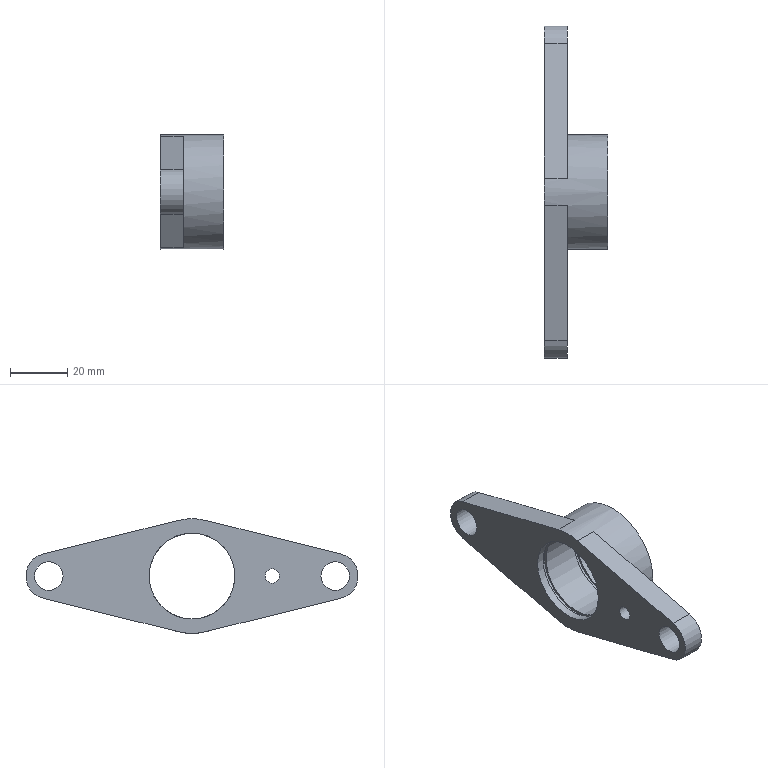Part | NX | features DATUM_CSYS 3, EXTRACT_FACE 2, EXTRUDE 2, RECT_GROOVE 2, Instance Feature 1, Mirror Feature 1, SKETCH 1 | 1 solid | 23 faces | box 22 x 116 x 40 mm | volume 25110 mm3 | plane 12 | cylinder 11 | commonest cylinder face diameters 30 x3 10 x2 16 x2 31.4 x2 5 x1 40 x1
STEP:
#1=CARTESIAN_POINT('',(22.,0.,15.));
#2=VERTEX_POINT('',#1);
#3=CARTESIAN_POINT('',(22.,0.,0.));
#4=DIRECTION('',(-1.,0.,0.));
#5=DIRECTION('',(0.,0.,1.));
#6=AXIS2_PLACEMENT_3D('',#3,#4,#5);
#7=CIRCLE('',#6,15.);
#8=EDGE_CURVE('',#2,#2,#7,.F.);
#9=ORIENTED_EDGE('',*,*,#8,.T.);
#10=EDGE_LOOP('',(#9));
#11=FACE_BOUND('',#10,.T.);
#12=CARTESIAN_POINT('',(19.2,0.,15.));
#13=VERTEX_POINT('',#12);
#14=CARTESIAN_POINT('',(19.2,0.,0.));
#15=DIRECTION('',(-1.,0.,0.));
#16=DIRECTION('',(0.,0.,1.));
#17=AXIS2_PLACEMENT_3D('',#14,#15,#16);
#18=CIRCLE('',#17,15.);
#19=EDGE_CURVE('',#13,#13,#18,.T.);
#20=ORIENTED_EDGE('',*,*,#19,.T.);
#21=EDGE_LOOP('',(#20));
#22=FACE_BOUND('',#21,.T.);
#23=CARTESIAN_POINT('',(8.,0.,0.));
#24=DIRECTION('',(-1.,0.,0.));
#25=DIRECTION('',(0.,0.,1.));
#26=AXIS2_PLACEMENT_3D('',#23,#24,#25);
#27=CYLINDRICAL_SURFACE('',#26,15.);
#28=ADVANCED_FACE('',(#11,#22),#27,.F.);
#29=CARTESIAN_POINT('',(0.,15.,0.));
#30=VERTEX_POINT('',#29);
#31=CARTESIAN_POINT('',(0.,0.,0.));
#32=DIRECTION('',(1.,0.,0.));
#33=DIRECTION('',(0.,1.,0.));
#34=AXIS2_PLACEMENT_3D('',#31,#32,#33);
#35=CIRCLE('',#34,15.);
#36=EDGE_CURVE('',#30,#30,#35,.T.);
#37=ORIENTED_EDGE('',*,*,#36,.F.);
#38=EDGE_LOOP('',(#37));
#39=FACE_BOUND('',#38,.T.);
#40=CARTESIAN_POINT('',(2.8,0.,-15.));
#41=VERTEX_POINT('',#40);
#42=CARTESIAN_POINT('',(2.8,0.,0.));
#43=DIRECTION('',(1.,0.,0.));
#44=DIRECTION('',(0.,0.,-1.));
#45=AXIS2_PLACEMENT_3D('',#42,#43,#44);
#46=CIRCLE('',#45,15.);
#47=EDGE_CURVE('',#41,#41,#46,.T.);
#48=ORIENTED_EDGE('',*,*,#47,.T.);
#49=EDGE_LOOP('',(#48));
#50=FACE_BOUND('',#49,.T.);
#51=CARTESIAN_POINT('',(8.,0.,0.));
#52=DIRECTION('',(-1.,0.,0.));
#53=DIRECTION('',(0.,0.,1.));
#54=AXIS2_PLACEMENT_3D('',#51,#52,#53);
#55=CYLINDRICAL_SURFACE('',#54,15.);
#56=ADVANCED_FACE('',(#39,#50),#55,.F.);
#57=CARTESIAN_POINT('',(8.,-25.5,0.));
#58=VERTEX_POINT('',#57);
#59=CARTESIAN_POINT('',(8.,-28.,0.));
#60=DIRECTION('',(1.,0.,0.));
#61=DIRECTION('',(0.,1.,0.));
#62=AXIS2_PLACEMENT_3D('',#59,#60,#61);
#63=CIRCLE('',#62,2.5);
#64=EDGE_CURVE('',#58,#58,#63,.T.);
#65=ORIENTED_EDGE('',*,*,#64,.F.);
#66=EDGE_LOOP('',(#65));
#67=FACE_BOUND('',#66,.T.);
#68=CARTESIAN_POINT('',(8.,-45.,0.));
#69=VERTEX_POINT('',#68);
#70=CARTESIAN_POINT('',(8.,-50.,0.));
#71=DIRECTION('',(1.,0.,0.));
#72=DIRECTION('',(0.,1.,0.));
#73=AXIS2_PLACEMENT_3D('',#70,#71,#72);
#74=CIRCLE('',#73,5.);
#75=EDGE_CURVE('',#69,#69,#74,.T.);
#76=ORIENTED_EDGE('',*,*,#75,.F.);
#77=EDGE_LOOP('',(#76));
#78=FACE_BOUND('',#77,.T.);
#79=CARTESIAN_POINT('',(8.,-4.8,19.415));
#80=VERTEX_POINT('',#79);
#81=CARTESIAN_POINT('',(8.,-4.8,-19.415));
#82=VERTEX_POINT('',#81);
#83=CARTESIAN_POINT('',(8.,0.,0.));
#84=DIRECTION('',(-1.,0.,0.));
#85=DIRECTION('',(0.,0.,1.));
#86=AXIS2_PLACEMENT_3D('',#83,#84,#85);
#87=CIRCLE('',#86,20.);
#88=EDGE_CURVE('',#80,#82,#87,.F.);
#89=ORIENTED_EDGE('',*,*,#88,.F.);
#90=CARTESIAN_POINT('',(8.,-51.92,7.766));
#91=VERTEX_POINT('',#90);
#92=CARTESIAN_POINT('',(8.,-51.92,7.766));
#93=DIRECTION('',(0.,0.9708,0.24));
#94=VECTOR('',#93,1000.);
#95=LINE('',#92,#94);
#96=EDGE_CURVE('',#91,#80,#95,.T.);
#97=ORIENTED_EDGE('',*,*,#96,.F.);
#98=CARTESIAN_POINT('',(8.,-51.92,-7.766));
#99=VERTEX_POINT('',#98);
#100=CARTESIAN_POINT('',(8.,-50.,0.));
#101=DIRECTION('',(-1.,0.,0.));
#102=DIRECTION('',(0.,1.,0.));
#103=AXIS2_PLACEMENT_3D('',#100,#101,#102);
#104=CIRCLE('',#103,8.);
#105=EDGE_CURVE('',#99,#91,#104,.T.);
#106=ORIENTED_EDGE('',*,*,#105,.F.);
#107=CARTESIAN_POINT('',(8.,-4.8,-19.415));
#108=DIRECTION('',(0.,-0.9708,0.24));
#109=VECTOR('',#108,1000.);
#110=LINE('',#107,#109);
#111=EDGE_CURVE('',#82,#99,#110,.T.);
#112=ORIENTED_EDGE('',*,*,#111,.F.);
#113=EDGE_LOOP('',(#89,#97,#106,#112));
#114=FACE_BOUND('',#113,.T.);
#115=CARTESIAN_POINT('',(8.,0.,0.));
#116=DIRECTION('',(-1.,0.,0.));
#117=DIRECTION('',(0.,0.,1.));
#118=AXIS2_PLACEMENT_3D('',#115,#116,#117);
#119=PLANE('',#118);
#120=ADVANCED_FACE('',(#67,#78,#114),#119,.F.);
#121=CARTESIAN_POINT('',(8.,45.,0.));
#122=VERTEX_POINT('',#121);
#123=CARTESIAN_POINT('',(8.,50.,0.));
#124=DIRECTION('',(-1.,0.,0.));
#125=DIRECTION('',(0.,-1.,0.));
#126=AXIS2_PLACEMENT_3D('',#123,#124,#125);
#127=CIRCLE('',#126,5.);
#128=EDGE_CURVE('',#122,#122,#127,.T.);
#129=ORIENTED_EDGE('',*,*,#128,.T.);
#130=EDGE_LOOP('',(#129));
#131=FACE_BOUND('',#130,.T.);
#132=CARTESIAN_POINT('',(8.,4.8,-19.415));
#133=VERTEX_POINT('',#132);
#134=CARTESIAN_POINT('',(8.,4.8,19.415));
#135=VERTEX_POINT('',#134);
#136=CARTESIAN_POINT('',(8.,0.,0.));
#137=DIRECTION('',(-1.,0.,0.));
#138=DIRECTION('',(0.,0.,1.));
#139=AXIS2_PLACEMENT_3D('',#136,#137,#138);
#140=CIRCLE('',#139,20.);
#141=EDGE_CURVE('',#133,#135,#140,.F.);
#142=ORIENTED_EDGE('',*,*,#141,.F.);
#143=CARTESIAN_POINT('',(8.,51.92,-7.766));
#144=VERTEX_POINT('',#143);
#145=CARTESIAN_POINT('',(8.,51.92,-7.766));
#146=DIRECTION('',(0.,-0.9708,-0.24));
#147=VECTOR('',#146,1000.);
#148=LINE('',#145,#147);
#149=EDGE_CURVE('',#144,#133,#148,.T.);
#150=ORIENTED_EDGE('',*,*,#149,.F.);
#151=CARTESIAN_POINT('',(8.,51.92,7.766));
#152=VERTEX_POINT('',#151);
#153=CARTESIAN_POINT('',(8.,50.,0.));
#154=DIRECTION('',(-1.,0.,0.));
#155=DIRECTION('',(0.,-1.,0.));
#156=AXIS2_PLACEMENT_3D('',#153,#154,#155);
#157=CIRCLE('',#156,8.);
#158=EDGE_CURVE('',#152,#144,#157,.T.);
#159=ORIENTED_EDGE('',*,*,#158,.F.);
#160=CARTESIAN_POINT('',(8.,4.8,19.415));
#161=DIRECTION('',(0.,0.9708,-0.24));
#162=VECTOR('',#161,1000.);
#163=LINE('',#160,#162);
#164=EDGE_CURVE('',#135,#152,#163,.T.);
#165=ORIENTED_EDGE('',*,*,#164,.F.);
#166=EDGE_LOOP('',(#142,#150,#159,#165));
#167=FACE_BOUND('',#166,.T.);
#168=CARTESIAN_POINT('',(8.,0.,0.));
#169=DIRECTION('',(-1.,0.,0.));
#170=DIRECTION('',(0.,0.,1.));
#171=AXIS2_PLACEMENT_3D('',#168,#169,#170);
#172=PLANE('',#171);
#173=ADVANCED_FACE('',(#131,#167),#172,.F.);
#174=CARTESIAN_POINT('',(0.,-51.92,7.766));
#175=VERTEX_POINT('',#174);
#176=CARTESIAN_POINT('',(0.,-4.8,19.415));
#177=VERTEX_POINT('',#176);
#178=CARTESIAN_POINT('',(0.,-51.92,7.766));
#179=DIRECTION('',(0.,0.9708,0.24));
#180=VECTOR('',#179,1000.);
#181=LINE('',#178,#180);
#182=EDGE_CURVE('',#175,#177,#181,.T.);
#183=ORIENTED_EDGE('',*,*,#182,.F.);
#184=CARTESIAN_POINT('',(8.,-51.92,7.766));
#185=DIRECTION('',(-1.,0.,0.));
#186=VECTOR('',#185,1000.);
#187=LINE('',#184,#186);
#188=EDGE_CURVE('',#91,#175,#187,.T.);
#189=ORIENTED_EDGE('',*,*,#188,.F.);
#190=ORIENTED_EDGE('',*,*,#96,.T.);
#191=CARTESIAN_POINT('',(8.,-4.8,19.415));
#192=DIRECTION('',(-1.,0.,0.));
#193=VECTOR('',#192,1000.);
#194=LINE('',#191,#193);
#195=EDGE_CURVE('',#80,#177,#194,.T.);
#196=ORIENTED_EDGE('',*,*,#195,.T.);
#197=EDGE_LOOP('',(#183,#189,#190,#196));
#198=FACE_BOUND('',#197,.T.);
#199=CARTESIAN_POINT('',(8.,-51.92,7.766));
#200=DIRECTION('',(0.,-0.24,0.9708));
#201=DIRECTION('',(0.,-0.9708,-0.24));
#202=AXIS2_PLACEMENT_3D('',#199,#200,#201);
#203=PLANE('',#202);
#204=ADVANCED_FACE('',(#198),#203,.T.);
#205=CARTESIAN_POINT('',(0.,4.8,19.415));
#206=VERTEX_POINT('',#205);
#207=CARTESIAN_POINT('',(0.,51.92,7.766));
#208=VERTEX_POINT('',#207);
#209=CARTESIAN_POINT('',(0.,4.8,19.415));
#210=DIRECTION('',(0.,0.9708,-0.24));
#211=VECTOR('',#210,1000.);
#212=LINE('',#209,#211);
#213=EDGE_CURVE('',#206,#208,#212,.T.);
#214=ORIENTED_EDGE('',*,*,#213,.F.);
#215=CARTESIAN_POINT('',(8.,4.8,19.415));
#216=DIRECTION('',(-1.,0.,0.));
#217=VECTOR('',#216,1000.);
#218=LINE('',#215,#217);
#219=EDGE_CURVE('',#135,#206,#218,.T.);
#220=ORIENTED_EDGE('',*,*,#219,.F.);
#221=ORIENTED_EDGE('',*,*,#164,.T.);
#222=CARTESIAN_POINT('',(8.,51.92,7.766));
#223=DIRECTION('',(-1.,0.,0.));
#224=VECTOR('',#223,1000.);
#225=LINE('',#222,#224);
#226=EDGE_CURVE('',#152,#208,#225,.T.);
#227=ORIENTED_EDGE('',*,*,#226,.T.);
#228=EDGE_LOOP('',(#214,#220,#221,#227));
#229=FACE_BOUND('',#228,.T.);
#230=CARTESIAN_POINT('',(8.,4.8,19.415));
#231=DIRECTION('',(0.,0.24,0.9708));
#232=DIRECTION('',(0.,-0.9708,0.24));
#233=AXIS2_PLACEMENT_3D('',#230,#231,#232);
#234=PLANE('',#233);
#235=ADVANCED_FACE('',(#229),#234,.T.);
#236=CARTESIAN_POINT('',(0.,51.92,-7.766));
#237=VERTEX_POINT('',#236);
#238=CARTESIAN_POINT('',(0.,50.,0.));
#239=DIRECTION('',(-1.,0.,0.));
#240=DIRECTION('',(0.,-1.,0.));
#241=AXIS2_PLACEMENT_3D('',#238,#239,#240);
#242=CIRCLE('',#241,8.);
#243=EDGE_CURVE('',#208,#237,#242,.T.);
#244=ORIENTED_EDGE('',*,*,#243,.F.);
#245=ORIENTED_EDGE('',*,*,#226,.F.);
#246=ORIENTED_EDGE('',*,*,#158,.T.);
#247=CARTESIAN_POINT('',(8.,51.92,-7.766));
#248=DIRECTION('',(-1.,0.,0.));
#249=VECTOR('',#248,1000.);
#250=LINE('',#247,#249);
#251=EDGE_CURVE('',#144,#237,#250,.T.);
#252=ORIENTED_EDGE('',*,*,#251,.T.);
#253=EDGE_LOOP('',(#244,#245,#246,#252));
#254=FACE_BOUND('',#253,.T.);
#255=CARTESIAN_POINT('',(8.,50.,0.));
#256=DIRECTION('',(-1.,0.,0.));
#257=DIRECTION('',(0.,0.,1.));
#258=AXIS2_PLACEMENT_3D('',#255,#256,#257);
#259=CYLINDRICAL_SURFACE('',#258,8.);
#260=ADVANCED_FACE('',(#254),#259,.T.);
#261=CARTESIAN_POINT('',(0.,4.8,-19.415));
#262=VERTEX_POINT('',#261);
#263=CARTESIAN_POINT('',(0.,51.92,-7.766));
#264=DIRECTION('',(0.,-0.9708,-0.24));
#265=VECTOR('',#264,1000.);
#266=LINE('',#263,#265);
#267=EDGE_CURVE('',#237,#262,#266,.T.);
#268=ORIENTED_EDGE('',*,*,#267,.F.);
#269=ORIENTED_EDGE('',*,*,#251,.F.);
#270=ORIENTED_EDGE('',*,*,#149,.T.);
#271=CARTESIAN_POINT('',(8.,4.8,-19.415));
#272=DIRECTION('',(-1.,0.,0.));
#273=VECTOR('',#272,1000.);
#274=LINE('',#271,#273);
#275=EDGE_CURVE('',#133,#262,#274,.T.);
#276=ORIENTED_EDGE('',*,*,#275,.T.);
#277=EDGE_LOOP('',(#268,#269,#270,#276));
#278=FACE_BOUND('',#277,.T.);
#279=CARTESIAN_POINT('',(8.,51.92,-7.766));
#280=DIRECTION('',(0.,0.24,-0.9708));
#281=DIRECTION('',(0.,0.9708,0.24));
#282=AXIS2_PLACEMENT_3D('',#279,#280,#281);
#283=PLANE('',#282);
#284=ADVANCED_FACE('',(#278),#283,.T.);
#285=CARTESIAN_POINT('',(0.,-4.8,-19.415));
#286=VERTEX_POINT('',#285);
#287=CARTESIAN_POINT('',(0.,0.,0.));
#288=DIRECTION('',(-1.,0.,0.));
#289=DIRECTION('',(0.,1.,0.));
#290=AXIS2_PLACEMENT_3D('',#287,#288,#289);
#291=CIRCLE('',#290,20.);
#292=EDGE_CURVE('',#262,#286,#291,.T.);
#293=ORIENTED_EDGE('',*,*,#292,.F.);
#294=ORIENTED_EDGE('',*,*,#275,.F.);
#295=ORIENTED_EDGE('',*,*,#141,.T.);
#296=ORIENTED_EDGE('',*,*,#219,.T.);
#297=CARTESIAN_POINT('',(0.,0.,0.));
#298=DIRECTION('',(-1.,0.,0.));
#299=DIRECTION('',(0.,1.,0.));
#300=AXIS2_PLACEMENT_3D('',#297,#298,#299);
#301=CIRCLE('',#300,20.);
#302=EDGE_CURVE('',#177,#206,#301,.T.);
#303=ORIENTED_EDGE('',*,*,#302,.F.);
#304=ORIENTED_EDGE('',*,*,#195,.F.);
#305=ORIENTED_EDGE('',*,*,#88,.T.);
#306=CARTESIAN_POINT('',(8.,-4.8,-19.415));
#307=DIRECTION('',(-1.,0.,0.));
#308=VECTOR('',#307,1000.);
#309=LINE('',#306,#308);
#310=EDGE_CURVE('',#82,#286,#309,.T.);
#311=ORIENTED_EDGE('',*,*,#310,.T.);
#312=EDGE_LOOP('',(#293,#294,#295,#296,#303,#304,#305,#311));
#313=FACE_BOUND('',#312,.T.);
#314=CARTESIAN_POINT('',(22.,0.,20.));
#315=VERTEX_POINT('',#314);
#316=CARTESIAN_POINT('',(22.,0.,0.));
#317=DIRECTION('',(-1.,0.,0.));
#318=DIRECTION('',(0.,0.,1.));
#319=AXIS2_PLACEMENT_3D('',#316,#317,#318);
#320=CIRCLE('',#319,20.);
#321=EDGE_CURVE('',#315,#315,#320,.F.);
#322=ORIENTED_EDGE('',*,*,#321,.F.);
#323=EDGE_LOOP('',(#322));
#324=FACE_BOUND('',#323,.T.);
#325=CARTESIAN_POINT('',(8.,0.,0.));
#326=DIRECTION('',(-1.,0.,0.));
#327=DIRECTION('',(0.,0.,1.));
#328=AXIS2_PLACEMENT_3D('',#325,#326,#327);
#329=CYLINDRICAL_SURFACE('',#328,20.);
#330=ADVANCED_FACE('',(#313,#324),#329,.T.);
#331=CARTESIAN_POINT('',(0.,-51.92,-7.766));
#332=VERTEX_POINT('',#331);
#333=CARTESIAN_POINT('',(0.,-4.8,-19.415));
#334=DIRECTION('',(0.,-0.9708,0.24));
#335=VECTOR('',#334,1000.);
#336=LINE('',#333,#335);
#337=EDGE_CURVE('',#286,#332,#336,.T.);
#338=ORIENTED_EDGE('',*,*,#337,.F.);
#339=ORIENTED_EDGE('',*,*,#310,.F.);
#340=ORIENTED_EDGE('',*,*,#111,.T.);
#341=CARTESIAN_POINT('',(8.,-51.92,-7.766));
#342=DIRECTION('',(-1.,0.,0.));
#343=VECTOR('',#342,1000.);
#344=LINE('',#341,#343);
#345=EDGE_CURVE('',#99,#332,#344,.T.);
#346=ORIENTED_EDGE('',*,*,#345,.T.);
#347=EDGE_LOOP('',(#338,#339,#340,#346));
#348=FACE_BOUND('',#347,.T.);
#349=CARTESIAN_POINT('',(8.,-4.8,-19.415));
#350=DIRECTION('',(0.,-0.24,-0.9708));
#351=DIRECTION('',(0.,0.9708,-0.24));
#352=AXIS2_PLACEMENT_3D('',#349,#350,#351);
#353=PLANE('',#352);
#354=ADVANCED_FACE('',(#348),#353,.T.);
#355=CARTESIAN_POINT('',(17.9,0.,15.));
#356=VERTEX_POINT('',#355);
#357=CARTESIAN_POINT('',(17.9,0.,0.));
#358=DIRECTION('',(-1.,0.,0.));
#359=DIRECTION('',(0.,0.,1.));
#360=AXIS2_PLACEMENT_3D('',#357,#358,#359);
#361=CIRCLE('',#360,15.);
#362=EDGE_CURVE('',#356,#356,#361,.T.);
#363=ORIENTED_EDGE('',*,*,#362,.F.);
#364=EDGE_LOOP('',(#363));
#365=FACE_BOUND('',#364,.T.);
#366=CARTESIAN_POINT('',(4.1,0.,-15.));
#367=VERTEX_POINT('',#366);
#368=CARTESIAN_POINT('',(4.1,0.,0.));
#369=DIRECTION('',(1.,0.,0.));
#370=DIRECTION('',(0.,0.,-1.));
#371=AXIS2_PLACEMENT_3D('',#368,#369,#370);
#372=CIRCLE('',#371,15.);
#373=EDGE_CURVE('',#367,#367,#372,.T.);
#374=ORIENTED_EDGE('',*,*,#373,.F.);
#375=EDGE_LOOP('',(#374));
#376=FACE_BOUND('',#375,.T.);
#377=CARTESIAN_POINT('',(8.,0.,0.));
#378=DIRECTION('',(-1.,0.,0.));
#379=DIRECTION('',(0.,0.,1.));
#380=AXIS2_PLACEMENT_3D('',#377,#378,#379);
#381=CYLINDRICAL_SURFACE('',#380,15.);
#382=ADVANCED_FACE('',(#365,#376),#381,.F.);
#383=ORIENTED_EDGE('',*,*,#64,.T.);
#384=EDGE_LOOP('',(#383));
#385=FACE_BOUND('',#384,.T.);
#386=CARTESIAN_POINT('',(0.,-25.5,0.));
#387=VERTEX_POINT('',#386);
#388=CARTESIAN_POINT('',(0.,-28.,0.));
#389=DIRECTION('',(1.,0.,0.));
#390=DIRECTION('',(0.,1.,0.));
#391=AXIS2_PLACEMENT_3D('',#388,#389,#390);
#392=CIRCLE('',#391,2.5);
#393=EDGE_CURVE('',#387,#387,#392,.T.);
#394=ORIENTED_EDGE('',*,*,#393,.F.);
#395=EDGE_LOOP('',(#394));
#396=FACE_BOUND('',#395,.T.);
#397=CARTESIAN_POINT('',(8.,-28.,0.));
#398=DIRECTION('',(-1.,0.,0.));
#399=DIRECTION('',(0.,0.,1.));
#400=AXIS2_PLACEMENT_3D('',#397,#398,#399);
#401=CYLINDRICAL_SURFACE('',#400,2.5);
#402=ADVANCED_FACE('',(#385,#396),#401,.F.);
#403=ORIENTED_EDGE('',*,*,#75,.T.);
#404=EDGE_LOOP('',(#403));
#405=FACE_BOUND('',#404,.T.);
#406=CARTESIAN_POINT('',(0.,-45.,0.));
#407=VERTEX_POINT('',#406);
#408=CARTESIAN_POINT('',(0.,-50.,0.));
#409=DIRECTION('',(1.,0.,0.));
#410=DIRECTION('',(0.,1.,0.));
#411=AXIS2_PLACEMENT_3D('',#408,#409,#410);
#412=CIRCLE('',#411,5.);
#413=EDGE_CURVE('',#407,#407,#412,.T.);
#414=ORIENTED_EDGE('',*,*,#413,.F.);
#415=EDGE_LOOP('',(#414));
#416=FACE_BOUND('',#415,.T.);
#417=CARTESIAN_POINT('',(8.,-50.,0.));
#418=DIRECTION('',(-1.,0.,0.));
#419=DIRECTION('',(0.,0.,1.));
#420=AXIS2_PLACEMENT_3D('',#417,#418,#419);
#421=CYLINDRICAL_SURFACE('',#420,5.);
#422=ADVANCED_FACE('',(#405,#416),#421,.F.);
#423=CARTESIAN_POINT('',(0.,-50.,0.));
#424=DIRECTION('',(-1.,0.,0.));
#425=DIRECTION('',(0.,1.,0.));
#426=AXIS2_PLACEMENT_3D('',#423,#424,#425);
#427=CIRCLE('',#426,8.);
#428=EDGE_CURVE('',#332,#175,#427,.T.);
#429=ORIENTED_EDGE('',*,*,#428,.F.);
#430=ORIENTED_EDGE('',*,*,#345,.F.);
#431=ORIENTED_EDGE('',*,*,#105,.T.);
#432=ORIENTED_EDGE('',*,*,#188,.T.);
#433=EDGE_LOOP('',(#429,#430,#431,#432));
#434=FACE_BOUND('',#433,.T.);
#435=CARTESIAN_POINT('',(8.,-50.,0.));
#436=DIRECTION('',(-1.,0.,0.));
#437=DIRECTION('',(0.,0.,1.));
#438=AXIS2_PLACEMENT_3D('',#435,#436,#437);
#439=CYLINDRICAL_SURFACE('',#438,8.);
#440=ADVANCED_FACE('',(#434),#439,.T.);
#441=ORIENTED_EDGE('',*,*,#128,.F.);
#442=EDGE_LOOP('',(#441));
#443=FACE_BOUND('',#442,.T.);
#444=CARTESIAN_POINT('',(0.,45.,0.));
#445=VERTEX_POINT('',#444);
#446=CARTESIAN_POINT('',(0.,50.,0.));
#447=DIRECTION('',(-1.,0.,0.));
#448=DIRECTION('',(0.,-1.,0.));
#449=AXIS2_PLACEMENT_3D('',#446,#447,#448);
#450=CIRCLE('',#449,5.);
#451=EDGE_CURVE('',#445,#445,#450,.T.);
#452=ORIENTED_EDGE('',*,*,#451,.T.);
#453=EDGE_LOOP('',(#452));
#454=FACE_BOUND('',#453,.T.);
#455=CARTESIAN_POINT('',(8.,50.,0.));
#456=DIRECTION('',(-1.,0.,0.));
#457=DIRECTION('',(0.,0.,1.));
#458=AXIS2_PLACEMENT_3D('',#455,#456,#457);
#459=CYLINDRICAL_SURFACE('',#458,5.);
#460=ADVANCED_FACE('',(#443,#454),#459,.F.);
#461=ORIENTED_EDGE('',*,*,#182,.T.);
#462=ORIENTED_EDGE('',*,*,#302,.T.);
#463=ORIENTED_EDGE('',*,*,#213,.T.);
#464=ORIENTED_EDGE('',*,*,#243,.T.);
#465=ORIENTED_EDGE('',*,*,#267,.T.);
#466=ORIENTED_EDGE('',*,*,#292,.T.);
#467=ORIENTED_EDGE('',*,*,#337,.T.);
#468=ORIENTED_EDGE('',*,*,#428,.T.);
#469=EDGE_LOOP('',(#461,#462,#463,#464,#465,#466,#467,#468));
#470=FACE_BOUND('',#469,.T.);
#471=ORIENTED_EDGE('',*,*,#413,.T.);
#472=EDGE_LOOP('',(#471));
#473=FACE_BOUND('',#472,.T.);
#474=ORIENTED_EDGE('',*,*,#393,.T.);
#475=EDGE_LOOP('',(#474));
#476=FACE_BOUND('',#475,.T.);
#477=ORIENTED_EDGE('',*,*,#36,.T.);
#478=EDGE_LOOP('',(#477));
#479=FACE_BOUND('',#478,.T.);
#480=ORIENTED_EDGE('',*,*,#451,.F.);
#481=EDGE_LOOP('',(#480));
#482=FACE_BOUND('',#481,.T.);
#483=CARTESIAN_POINT('',(0.,0.,0.));
#484=DIRECTION('',(-1.,0.,0.));
#485=DIRECTION('',(0.,0.,1.));
#486=AXIS2_PLACEMENT_3D('',#483,#484,#485);
#487=PLANE('',#486);
#488=ADVANCED_FACE('',(#470,#473,#476,#479,#482),#487,.T.);
#489=ORIENTED_EDGE('',*,*,#8,.F.);
#490=EDGE_LOOP('',(#489));
#491=FACE_BOUND('',#490,.T.);
#492=ORIENTED_EDGE('',*,*,#321,.T.);
#493=EDGE_LOOP('',(#492));
#494=FACE_BOUND('',#493,.T.);
#495=CARTESIAN_POINT('',(22.,0.,0.));
#496=DIRECTION('',(-1.,0.,0.));
#497=DIRECTION('',(0.,0.,1.));
#498=AXIS2_PLACEMENT_3D('',#495,#496,#497);
#499=PLANE('',#498);
#500=ADVANCED_FACE('',(#491,#494),#499,.F.);
#501=CARTESIAN_POINT('',(4.1,0.,-15.7));
#502=VERTEX_POINT('',#501);
#503=CARTESIAN_POINT('',(4.1,0.,0.));
#504=DIRECTION('',(1.,0.,0.));
#505=DIRECTION('',(0.,0.,-1.));
#506=AXIS2_PLACEMENT_3D('',#503,#504,#505);
#507=CIRCLE('',#506,15.7);
#508=EDGE_CURVE('',#502,#502,#507,.F.);
#509=ORIENTED_EDGE('',*,*,#508,.F.);
#510=EDGE_LOOP('',(#509));
#511=FACE_BOUND('',#510,.T.);
#512=CARTESIAN_POINT('',(2.8,0.,-15.7));
#513=VERTEX_POINT('',#512);
#514=CARTESIAN_POINT('',(2.8,0.,0.));
#515=DIRECTION('',(1.,0.,0.));
#516=DIRECTION('',(0.,0.,-1.));
#517=AXIS2_PLACEMENT_3D('',#514,#515,#516);
#518=CIRCLE('',#517,15.7);
#519=EDGE_CURVE('',#513,#513,#518,.F.);
#520=ORIENTED_EDGE('',*,*,#519,.T.);
#521=EDGE_LOOP('',(#520));
#522=FACE_BOUND('',#521,.T.);
#523=CARTESIAN_POINT('',(3.45,0.,0.));
#524=DIRECTION('',(1.,0.,0.));
#525=DIRECTION('',(0.,0.,-1.));
#526=AXIS2_PLACEMENT_3D('',#523,#524,#525);
#527=CYLINDRICAL_SURFACE('',#526,15.7);
#528=ADVANCED_FACE('',(#511,#522),#527,.F.);
#529=ORIENTED_EDGE('',*,*,#47,.F.);
#530=EDGE_LOOP('',(#529));
#531=FACE_BOUND('',#530,.T.);
#532=ORIENTED_EDGE('',*,*,#519,.F.);
#533=EDGE_LOOP('',(#532));
#534=FACE_BOUND('',#533,.T.);
#535=CARTESIAN_POINT('',(2.8,0.,0.));
#536=DIRECTION('',(1.,0.,0.));
#537=DIRECTION('',(0.,0.,-1.));
#538=AXIS2_PLACEMENT_3D('',#535,#536,#537);
#539=PLANE('',#538);
#540=ADVANCED_FACE('',(#531,#534),#539,.T.);
#541=ORIENTED_EDGE('',*,*,#373,.T.);
#542=EDGE_LOOP('',(#541));
#543=FACE_BOUND('',#542,.T.);
#544=ORIENTED_EDGE('',*,*,#508,.T.);
#545=EDGE_LOOP('',(#544));
#546=FACE_BOUND('',#545,.T.);
#547=CARTESIAN_POINT('',(4.1,0.,0.));
#548=DIRECTION('',(1.,0.,0.));
#549=DIRECTION('',(0.,0.,-1.));
#550=AXIS2_PLACEMENT_3D('',#547,#548,#549);
#551=PLANE('',#550);
#552=ADVANCED_FACE('',(#543,#546),#551,.F.);
#553=CARTESIAN_POINT('',(17.9,0.,15.7));
#554=VERTEX_POINT('',#553);
#555=CARTESIAN_POINT('',(17.9,0.,0.));
#556=DIRECTION('',(-1.,0.,0.));
#557=DIRECTION('',(0.,0.,1.));
#558=AXIS2_PLACEMENT_3D('',#555,#556,#557);
#559=CIRCLE('',#558,15.7);
#560=EDGE_CURVE('',#554,#554,#559,.T.);
#561=ORIENTED_EDGE('',*,*,#560,.T.);
#562=EDGE_LOOP('',(#561));
#563=FACE_BOUND('',#562,.T.);
#564=CARTESIAN_POINT('',(19.2,0.,15.7));
#565=VERTEX_POINT('',#564);
#566=CARTESIAN_POINT('',(19.2,0.,0.));
#567=DIRECTION('',(-1.,0.,0.));
#568=DIRECTION('',(0.,0.,1.));
#569=AXIS2_PLACEMENT_3D('',#566,#567,#568);
#570=CIRCLE('',#569,15.7);
#571=EDGE_CURVE('',#565,#565,#570,.T.);
#572=ORIENTED_EDGE('',*,*,#571,.F.);
#573=EDGE_LOOP('',(#572));
#574=FACE_BOUND('',#573,.T.);
#575=CARTESIAN_POINT('',(18.55,0.,0.));
#576=DIRECTION('',(-1.,0.,0.));
#577=DIRECTION('',(0.,0.,1.));
#578=AXIS2_PLACEMENT_3D('',#575,#576,#577);
#579=CYLINDRICAL_SURFACE('',#578,15.7);
#580=ADVANCED_FACE('',(#563,#574),#579,.F.);
#581=ORIENTED_EDGE('',*,*,#19,.F.);
#582=EDGE_LOOP('',(#581));
#583=FACE_BOUND('',#582,.T.);
#584=ORIENTED_EDGE('',*,*,#571,.T.);
#585=EDGE_LOOP('',(#584));
#586=FACE_BOUND('',#585,.T.);
#587=CARTESIAN_POINT('',(19.2,0.,0.));
#588=DIRECTION('',(-1.,0.,0.));
#589=DIRECTION('',(0.,0.,1.));
#590=AXIS2_PLACEMENT_3D('',#587,#588,#589);
#591=PLANE('',#590);
#592=ADVANCED_FACE('',(#583,#586),#591,.T.);
#593=ORIENTED_EDGE('',*,*,#362,.T.);
#594=EDGE_LOOP('',(#593));
#595=FACE_BOUND('',#594,.T.);
#596=ORIENTED_EDGE('',*,*,#560,.F.);
#597=EDGE_LOOP('',(#596));
#598=FACE_BOUND('',#597,.T.);
#599=CARTESIAN_POINT('',(17.9,0.,0.));
#600=DIRECTION('',(-1.,0.,0.));
#601=DIRECTION('',(0.,0.,1.));
#602=AXIS2_PLACEMENT_3D('',#599,#600,#601);
#603=PLANE('',#602);
#604=ADVANCED_FACE('',(#595,#598),#603,.F.);
#605=CLOSED_SHELL('',(#28,#56,#120,#173,#204,#235,#260,#284,#330,#354,#382,#402,#422,#440,#460,#488,#500,#528,#540,#552,#580,#592,#604));
#606=MANIFOLD_SOLID_BREP('',#605);
#607=(LENGTH_UNIT()NAMED_UNIT(*)SI_UNIT(.MILLI.,.METRE.));
#608=UNCERTAINTY_MEASURE_WITH_UNIT(LENGTH_MEASURE(0.00001),#607,'','');
#609=(NAMED_UNIT(*)PLANE_ANGLE_UNIT()SI_UNIT($,.RADIAN.));
#610=(NAMED_UNIT(*)SI_UNIT($,.STERADIAN.)SOLID_ANGLE_UNIT());
#611=(GEOMETRIC_REPRESENTATION_CONTEXT(3)GLOBAL_UNCERTAINTY_ASSIGNED_CONTEXT((#608))GLOBAL_UNIT_ASSIGNED_CONTEXT((#607,#609,#610))REPRESENTATION_CONTEXT('',''));
#612=ADVANCED_BREP_SHAPE_REPRESENTATION('',(#606),#611);